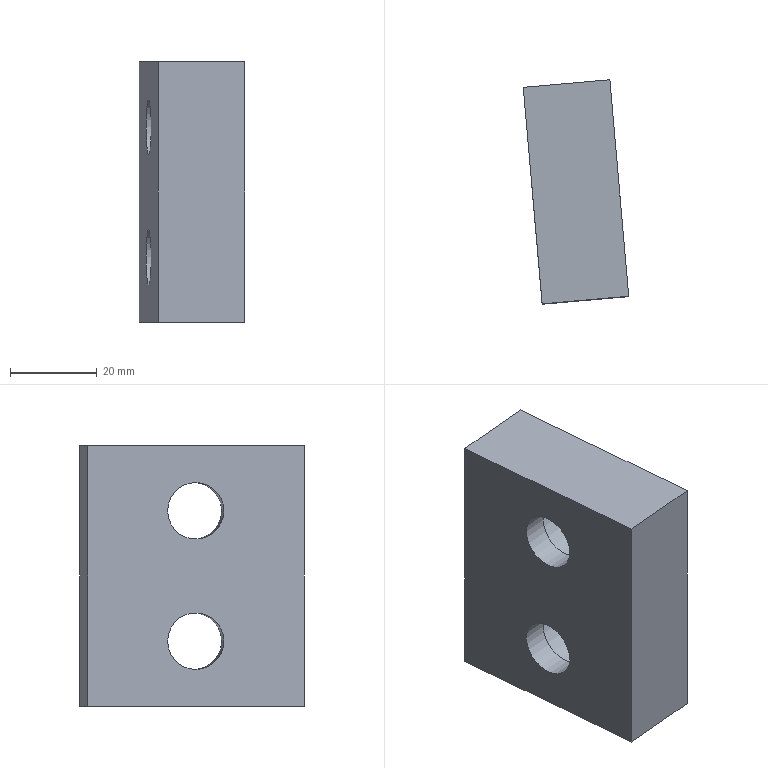Part | NX | features solid 2 | 1 solid | 12 faces | box 24.282 x 51.553 x 60 mm | volume 49611 mm3 | plane 8 | cylinder 4 | commonest cylinder face diameters 13 x2 20 x2
STEP:
#1=CARTESIAN_POINT('',(721.065,650.32,-295.));
#2=VERTEX_POINT('',#1);
#3=CARTESIAN_POINT('',(740.989,652.063,-295.));
#4=VERTEX_POINT('',#3);
#5=CARTESIAN_POINT('',(721.065,650.32,-295.));
#6=DIRECTION('',(0.9962,0.08716,0.));
#7=VECTOR('',#6,1000.);
#8=LINE('',#5,#7);
#9=EDGE_CURVE('',#2,#4,#8,.T.);
#10=ORIENTED_EDGE('',*,*,#9,.F.);
#11=CARTESIAN_POINT('',(716.707,700.129,-295.));
#12=VERTEX_POINT('',#11);
#13=CARTESIAN_POINT('',(721.065,650.32,-295.));
#14=DIRECTION('',(-0.08716,0.9962,0.));
#15=VECTOR('',#14,1000.);
#16=LINE('',#13,#15);
#17=EDGE_CURVE('',#2,#12,#16,.T.);
#18=ORIENTED_EDGE('',*,*,#17,.T.);
#19=CARTESIAN_POINT('',(736.631,701.872,-295.));
#20=VERTEX_POINT('',#19);
#21=CARTESIAN_POINT('',(716.707,700.129,-295.));
#22=DIRECTION('',(0.9962,0.08716,0.));
#23=VECTOR('',#22,1000.);
#24=LINE('',#21,#23);
#25=EDGE_CURVE('',#12,#20,#24,.T.);
#26=ORIENTED_EDGE('',*,*,#25,.T.);
#27=CARTESIAN_POINT('',(740.989,652.063,-295.));
#28=DIRECTION('',(-0.08716,0.9962,0.));
#29=VECTOR('',#28,1000.);
#30=LINE('',#27,#29);
#31=EDGE_CURVE('',#4,#20,#30,.T.);
#32=ORIENTED_EDGE('',*,*,#31,.F.);
#33=EDGE_LOOP('',(#10,#18,#26,#32));
#34=FACE_BOUND('',#33,.T.);
#35=CARTESIAN_POINT('',(721.065,650.32,-295.));
#36=DIRECTION('',(0.,0.,-1.));
#37=DIRECTION('',(-0.08716,0.9962,0.));
#38=AXIS2_PLACEMENT_3D('',#35,#36,#37);
#39=PLANE('',#38);
#40=ADVANCED_FACE('',(#34),#39,.T.);
#41=ORIENTED_EDGE('',*,*,#25,.F.);
#42=CARTESIAN_POINT('',(716.707,700.129,-235.));
#43=VERTEX_POINT('',#42);
#44=CARTESIAN_POINT('',(716.707,700.129,-295.));
#45=DIRECTION('',(0.,0.,1.));
#46=VECTOR('',#45,1000.);
#47=LINE('',#44,#46);
#48=EDGE_CURVE('',#12,#43,#47,.T.);
#49=ORIENTED_EDGE('',*,*,#48,.T.);
#50=CARTESIAN_POINT('',(736.631,701.872,-235.));
#51=VERTEX_POINT('',#50);
#52=CARTESIAN_POINT('',(716.707,700.129,-235.));
#53=DIRECTION('',(0.9962,0.08716,0.));
#54=VECTOR('',#53,1000.);
#55=LINE('',#52,#54);
#56=EDGE_CURVE('',#43,#51,#55,.T.);
#57=ORIENTED_EDGE('',*,*,#56,.T.);
#58=CARTESIAN_POINT('',(736.631,701.872,-295.));
#59=DIRECTION('',(0.,0.,1.));
#60=VECTOR('',#59,1000.);
#61=LINE('',#58,#60);
#62=EDGE_CURVE('',#20,#51,#61,.T.);
#63=ORIENTED_EDGE('',*,*,#62,.F.);
#64=EDGE_LOOP('',(#41,#49,#57,#63));
#65=FACE_BOUND('',#64,.T.);
#66=CARTESIAN_POINT('',(716.707,700.129,-295.));
#67=DIRECTION('',(-0.08716,0.9962,0.));
#68=DIRECTION('',(0.,0.,1.));
#69=AXIS2_PLACEMENT_3D('',#66,#67,#68);
#70=PLANE('',#69);
#71=ADVANCED_FACE('',(#65),#70,.T.);
#72=ORIENTED_EDGE('',*,*,#56,.F.);
#73=CARTESIAN_POINT('',(721.065,650.32,-235.));
#74=VERTEX_POINT('',#73);
#75=CARTESIAN_POINT('',(721.065,650.32,-235.));
#76=DIRECTION('',(-0.08716,0.9962,0.));
#77=VECTOR('',#76,1000.);
#78=LINE('',#75,#77);
#79=EDGE_CURVE('',#74,#43,#78,.T.);
#80=ORIENTED_EDGE('',*,*,#79,.F.);
#81=CARTESIAN_POINT('',(740.989,652.063,-235.));
#82=VERTEX_POINT('',#81);
#83=CARTESIAN_POINT('',(721.065,650.32,-235.));
#84=DIRECTION('',(0.9962,0.08716,0.));
#85=VECTOR('',#84,1000.);
#86=LINE('',#83,#85);
#87=EDGE_CURVE('',#74,#82,#86,.T.);
#88=ORIENTED_EDGE('',*,*,#87,.T.);
#89=CARTESIAN_POINT('',(740.989,652.063,-235.));
#90=DIRECTION('',(-0.08716,0.9962,0.));
#91=VECTOR('',#90,1000.);
#92=LINE('',#89,#91);
#93=EDGE_CURVE('',#82,#51,#92,.T.);
#94=ORIENTED_EDGE('',*,*,#93,.T.);
#95=EDGE_LOOP('',(#72,#80,#88,#94));
#96=FACE_BOUND('',#95,.T.);
#97=CARTESIAN_POINT('',(721.065,650.32,-235.));
#98=DIRECTION('',(0.,0.,-1.));
#99=DIRECTION('',(-0.08716,0.9962,0.));
#100=AXIS2_PLACEMENT_3D('',#97,#98,#99);
#101=PLANE('',#100);
#102=ADVANCED_FACE('',(#96),#101,.F.);
#103=CARTESIAN_POINT('',(721.065,650.32,-295.));
#104=DIRECTION('',(0.,0.,1.));
#105=VECTOR('',#104,1000.);
#106=LINE('',#103,#105);
#107=EDGE_CURVE('',#2,#74,#106,.T.);
#108=ORIENTED_EDGE('',*,*,#107,.F.);
#109=ORIENTED_EDGE('',*,*,#9,.T.);
#110=CARTESIAN_POINT('',(740.989,652.063,-295.));
#111=DIRECTION('',(0.,0.,1.));
#112=VECTOR('',#111,1000.);
#113=LINE('',#110,#112);
#114=EDGE_CURVE('',#4,#82,#113,.T.);
#115=ORIENTED_EDGE('',*,*,#114,.T.);
#116=ORIENTED_EDGE('',*,*,#87,.F.);
#117=EDGE_LOOP('',(#108,#109,#115,#116));
#118=FACE_BOUND('',#117,.T.);
#119=CARTESIAN_POINT('',(721.065,650.32,-295.));
#120=DIRECTION('',(-0.08716,0.9962,0.));
#121=DIRECTION('',(0.,0.,1.));
#122=AXIS2_PLACEMENT_3D('',#119,#120,#121);
#123=PLANE('',#122);
#124=ADVANCED_FACE('',(#118),#123,.F.);
#125=CARTESIAN_POINT('',(739.681,667.006,-250.));
#126=VERTEX_POINT('',#125);
#127=CARTESIAN_POINT('',(738.81,676.968,-250.));
#128=DIRECTION('',(-0.9962,-0.08716,0.));
#129=DIRECTION('',(0.08716,-0.9962,0.));
#130=AXIS2_PLACEMENT_3D('',#127,#128,#129);
#131=CIRCLE('',#130,10.);
#132=EDGE_CURVE('',#126,#126,#131,.T.);
#133=ORIENTED_EDGE('',*,*,#132,.T.);
#134=EDGE_LOOP('',(#133));
#135=FACE_BOUND('',#134,.T.);
#136=CARTESIAN_POINT('',(739.681,667.006,-280.));
#137=VERTEX_POINT('',#136);
#138=CARTESIAN_POINT('',(738.81,676.968,-280.));
#139=DIRECTION('',(-0.9962,-0.08716,0.));
#140=DIRECTION('',(0.08716,-0.9962,0.));
#141=AXIS2_PLACEMENT_3D('',#138,#139,#140);
#142=CIRCLE('',#141,10.);
#143=EDGE_CURVE('',#137,#137,#142,.T.);
#144=ORIENTED_EDGE('',*,*,#143,.T.);
#145=EDGE_LOOP('',(#144));
#146=FACE_BOUND('',#145,.T.);
#147=ORIENTED_EDGE('',*,*,#93,.F.);
#148=ORIENTED_EDGE('',*,*,#114,.F.);
#149=ORIENTED_EDGE('',*,*,#31,.T.);
#150=ORIENTED_EDGE('',*,*,#62,.T.);
#151=EDGE_LOOP('',(#147,#148,#149,#150));
#152=FACE_BOUND('',#151,.T.);
#153=CARTESIAN_POINT('',(740.989,652.063,-295.));
#154=DIRECTION('',(0.9962,0.08716,0.));
#155=DIRECTION('',(-0.08716,0.9962,0.));
#156=AXIS2_PLACEMENT_3D('',#153,#154,#155);
#157=PLANE('',#156);
#158=ADVANCED_FACE('',(#135,#146,#152),#157,.T.);
#159=CARTESIAN_POINT('',(718.319,681.7,-280.));
#160=VERTEX_POINT('',#159);
#161=CARTESIAN_POINT('',(718.886,675.224,-280.));
#162=DIRECTION('',(0.9962,0.08716,0.));
#163=DIRECTION('',(-0.08716,0.9962,0.));
#164=AXIS2_PLACEMENT_3D('',#161,#162,#163);
#165=CIRCLE('',#164,6.5);
#166=EDGE_CURVE('',#160,#160,#165,.T.);
#167=ORIENTED_EDGE('',*,*,#166,.T.);
#168=EDGE_LOOP('',(#167));
#169=FACE_BOUND('',#168,.T.);
#170=CARTESIAN_POINT('',(718.319,681.7,-250.));
#171=VERTEX_POINT('',#170);
#172=CARTESIAN_POINT('',(718.886,675.224,-250.));
#173=DIRECTION('',(0.9962,0.08716,0.));
#174=DIRECTION('',(-0.08716,0.9962,0.));
#175=AXIS2_PLACEMENT_3D('',#172,#173,#174);
#176=CIRCLE('',#175,6.5);
#177=EDGE_CURVE('',#171,#171,#176,.T.);
#178=ORIENTED_EDGE('',*,*,#177,.T.);
#179=EDGE_LOOP('',(#178));
#180=FACE_BOUND('',#179,.T.);
#181=ORIENTED_EDGE('',*,*,#79,.T.);
#182=ORIENTED_EDGE('',*,*,#48,.F.);
#183=ORIENTED_EDGE('',*,*,#17,.F.);
#184=ORIENTED_EDGE('',*,*,#107,.T.);
#185=EDGE_LOOP('',(#181,#182,#183,#184));
#186=FACE_BOUND('',#185,.T.);
#187=CARTESIAN_POINT('',(721.065,650.32,-295.));
#188=DIRECTION('',(0.9962,0.08716,0.));
#189=DIRECTION('',(-0.08716,0.9962,0.));
#190=AXIS2_PLACEMENT_3D('',#187,#188,#189);
#191=PLANE('',#190);
#192=ADVANCED_FACE('',(#169,#180,#186),#191,.F.);
#193=CARTESIAN_POINT('',(725.43,669.272,-280.));
#194=VERTEX_POINT('',#193);
#195=CARTESIAN_POINT('',(724.863,675.747,-280.));
#196=DIRECTION('',(-0.9962,-0.08716,0.));
#197=DIRECTION('',(0.08716,-0.9962,0.));
#198=AXIS2_PLACEMENT_3D('',#195,#196,#197);
#199=CIRCLE('',#198,6.5);
#200=EDGE_CURVE('',#194,#194,#199,.T.);
#201=ORIENTED_EDGE('',*,*,#200,.T.);
#202=EDGE_LOOP('',(#201));
#203=FACE_BOUND('',#202,.T.);
#204=CARTESIAN_POINT('',(725.735,665.785,-280.));
#205=VERTEX_POINT('',#204);
#206=CARTESIAN_POINT('',(724.863,675.747,-280.));
#207=DIRECTION('',(-0.9962,-0.08716,0.));
#208=DIRECTION('',(0.08716,-0.9962,0.));
#209=AXIS2_PLACEMENT_3D('',#206,#207,#208);
#210=CIRCLE('',#209,10.);
#211=EDGE_CURVE('',#205,#205,#210,.T.);
#212=ORIENTED_EDGE('',*,*,#211,.F.);
#213=EDGE_LOOP('',(#212));
#214=FACE_BOUND('',#213,.T.);
#215=CARTESIAN_POINT('',(724.863,675.747,-280.));
#216=DIRECTION('',(-0.9962,-0.08716,0.));
#217=DIRECTION('',(0.08716,-0.9962,0.));
#218=AXIS2_PLACEMENT_3D('',#215,#216,#217);
#219=PLANE('',#218);
#220=ADVANCED_FACE('',(#203,#214),#219,.F.);
#221=ORIENTED_EDGE('',*,*,#211,.T.);
#222=EDGE_LOOP('',(#221));
#223=FACE_BOUND('',#222,.T.);
#224=ORIENTED_EDGE('',*,*,#143,.F.);
#225=EDGE_LOOP('',(#224));
#226=FACE_BOUND('',#225,.T.);
#227=CARTESIAN_POINT('',(738.81,676.968,-280.));
#228=DIRECTION('',(-0.9962,-0.08716,0.));
#229=DIRECTION('',(0.08716,-0.9962,0.));
#230=AXIS2_PLACEMENT_3D('',#227,#228,#229);
#231=CYLINDRICAL_SURFACE('',#230,10.);
#232=ADVANCED_FACE('',(#223,#226),#231,.F.);
#233=CARTESIAN_POINT('',(725.43,669.272,-250.));
#234=VERTEX_POINT('',#233);
#235=CARTESIAN_POINT('',(724.863,675.747,-250.));
#236=DIRECTION('',(-0.9962,-0.08716,0.));
#237=DIRECTION('',(0.08716,-0.9962,0.));
#238=AXIS2_PLACEMENT_3D('',#235,#236,#237);
#239=CIRCLE('',#238,6.5);
#240=EDGE_CURVE('',#234,#234,#239,.T.);
#241=ORIENTED_EDGE('',*,*,#240,.T.);
#242=EDGE_LOOP('',(#241));
#243=FACE_BOUND('',#242,.T.);
#244=CARTESIAN_POINT('',(725.735,665.785,-250.));
#245=VERTEX_POINT('',#244);
#246=CARTESIAN_POINT('',(724.863,675.747,-250.));
#247=DIRECTION('',(-0.9962,-0.08716,0.));
#248=DIRECTION('',(0.08716,-0.9962,0.));
#249=AXIS2_PLACEMENT_3D('',#246,#247,#248);
#250=CIRCLE('',#249,10.);
#251=EDGE_CURVE('',#245,#245,#250,.T.);
#252=ORIENTED_EDGE('',*,*,#251,.F.);
#253=EDGE_LOOP('',(#252));
#254=FACE_BOUND('',#253,.T.);
#255=CARTESIAN_POINT('',(724.863,675.747,-250.));
#256=DIRECTION('',(-0.9962,-0.08716,0.));
#257=DIRECTION('',(0.08716,-0.9962,0.));
#258=AXIS2_PLACEMENT_3D('',#255,#256,#257);
#259=PLANE('',#258);
#260=ADVANCED_FACE('',(#243,#254),#259,.F.);
#261=ORIENTED_EDGE('',*,*,#251,.T.);
#262=EDGE_LOOP('',(#261));
#263=FACE_BOUND('',#262,.T.);
#264=ORIENTED_EDGE('',*,*,#132,.F.);
#265=EDGE_LOOP('',(#264));
#266=FACE_BOUND('',#265,.T.);
#267=CARTESIAN_POINT('',(738.81,676.968,-250.));
#268=DIRECTION('',(-0.9962,-0.08716,0.));
#269=DIRECTION('',(0.08716,-0.9962,0.));
#270=AXIS2_PLACEMENT_3D('',#267,#268,#269);
#271=CYLINDRICAL_SURFACE('',#270,10.);
#272=ADVANCED_FACE('',(#263,#266),#271,.F.);
#273=ORIENTED_EDGE('',*,*,#240,.F.);
#274=EDGE_LOOP('',(#273));
#275=FACE_BOUND('',#274,.T.);
#276=ORIENTED_EDGE('',*,*,#177,.F.);
#277=EDGE_LOOP('',(#276));
#278=FACE_BOUND('',#277,.T.);
#279=CARTESIAN_POINT('',(724.863,675.747,-250.));
#280=DIRECTION('',(-0.9962,-0.08716,0.));
#281=DIRECTION('',(0.08716,-0.9962,0.));
#282=AXIS2_PLACEMENT_3D('',#279,#280,#281);
#283=CYLINDRICAL_SURFACE('',#282,6.5);
#284=ADVANCED_FACE('',(#275,#278),#283,.F.);
#285=ORIENTED_EDGE('',*,*,#200,.F.);
#286=EDGE_LOOP('',(#285));
#287=FACE_BOUND('',#286,.T.);
#288=ORIENTED_EDGE('',*,*,#166,.F.);
#289=EDGE_LOOP('',(#288));
#290=FACE_BOUND('',#289,.T.);
#291=CARTESIAN_POINT('',(724.863,675.747,-280.));
#292=DIRECTION('',(-0.9962,-0.08716,0.));
#293=DIRECTION('',(0.08716,-0.9962,0.));
#294=AXIS2_PLACEMENT_3D('',#291,#292,#293);
#295=CYLINDRICAL_SURFACE('',#294,6.5);
#296=ADVANCED_FACE('',(#287,#290),#295,.F.);
#297=CLOSED_SHELL('',(#40,#71,#102,#124,#158,#192,#220,#232,#260,#272,#284,#296));
#298=MANIFOLD_SOLID_BREP('',#297);
#299=(LENGTH_UNIT()NAMED_UNIT(*)SI_UNIT(.MILLI.,.METRE.));
#300=UNCERTAINTY_MEASURE_WITH_UNIT(LENGTH_MEASURE(0.00001),#299,'','');
#301=(NAMED_UNIT(*)PLANE_ANGLE_UNIT()SI_UNIT($,.RADIAN.));
#302=(NAMED_UNIT(*)SI_UNIT($,.STERADIAN.)SOLID_ANGLE_UNIT());
#303=(GEOMETRIC_REPRESENTATION_CONTEXT(3)GLOBAL_UNCERTAINTY_ASSIGNED_CONTEXT((#300))GLOBAL_UNIT_ASSIGNED_CONTEXT((#299,#301,#302))REPRESENTATION_CONTEXT('',''));
#304=ADVANCED_BREP_SHAPE_REPRESENTATION('',(#298),#303);